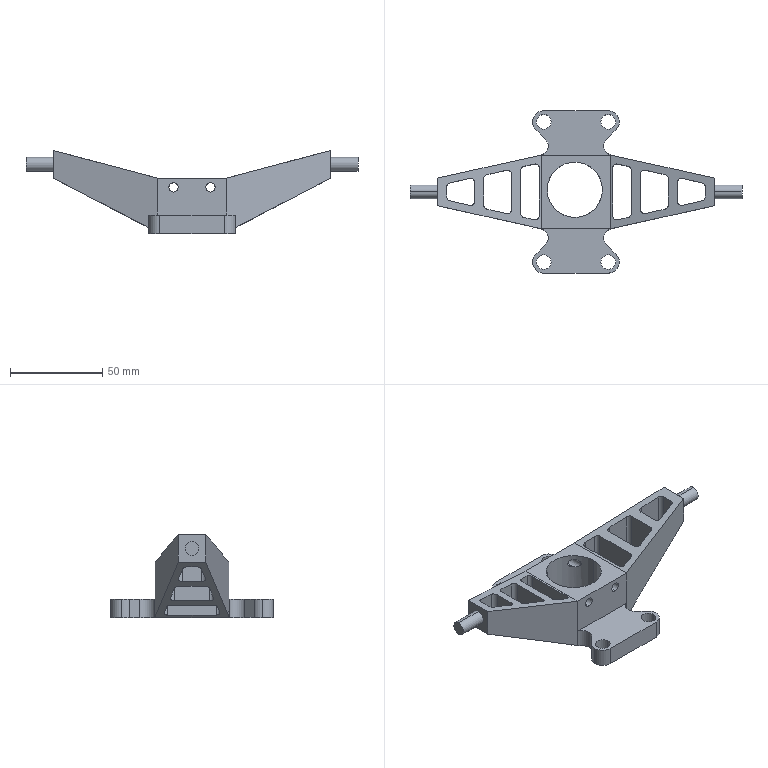Part | NX | features BREP 2 | 2 solids | 116 faces | box 180 x 88 x 45 mm | volume 75635 mm3 | cylinder 58 | plane 58 | commonest cylinder face diameters 4.345 x20 5 x8 8 x8 10 x6 12 x6 4 x4